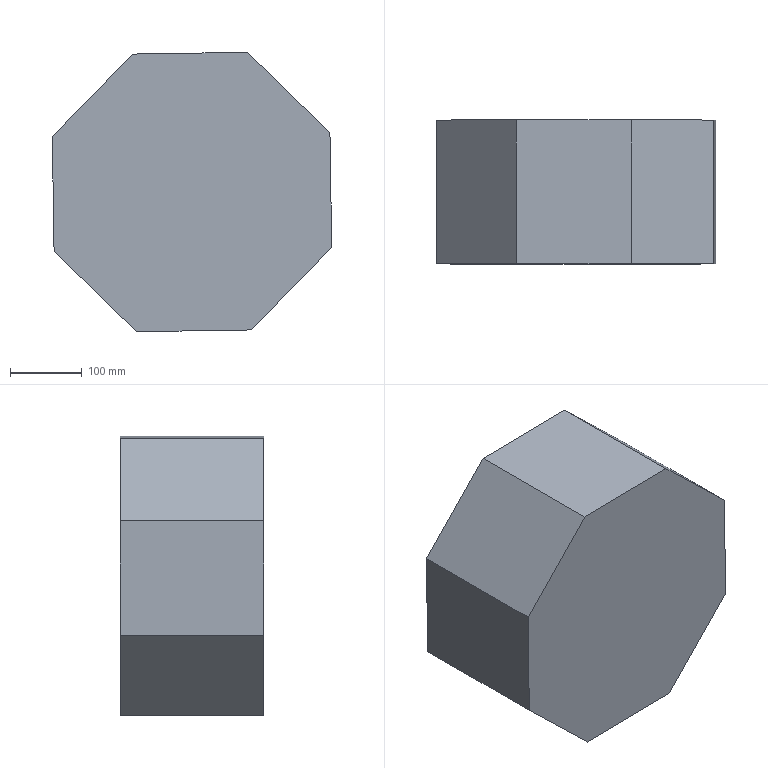Part | STEP file | octahedron 160 193.step.STEP | 1 solid | 10 faces | box 388.677 x 200 x 388.677 mm | volume 24721547 mm3 | plane 10
STEP:
#1=CARTESIAN_POINT('',(77.035,0.,194.339));
#2=VERTEX_POINT('',#1);
#3=CARTESIAN_POINT('',(191.89,0.,82.946));
#4=VERTEX_POINT('',#3);
#5=CARTESIAN_POINT('',(77.035,0.,194.339));
#6=DIRECTION('',(0.7178,0.,-0.6962));
#7=VECTOR('',#6,1000.);
#8=LINE('',#5,#7);
#9=EDGE_CURVE('',#2,#4,#8,.T.);
#10=ORIENTED_EDGE('',*,*,#9,.T.);
#11=CARTESIAN_POINT('',(191.89,200.,82.946));
#12=VERTEX_POINT('',#11);
#13=CARTESIAN_POINT('',(191.89,200.,82.946));
#14=DIRECTION('',(0.,-1.,0.));
#15=VECTOR('',#14,1000.);
#16=LINE('',#13,#15);
#17=EDGE_CURVE('',#12,#4,#16,.T.);
#18=ORIENTED_EDGE('',*,*,#17,.F.);
#19=CARTESIAN_POINT('',(77.035,200.,194.339));
#20=VERTEX_POINT('',#19);
#21=CARTESIAN_POINT('',(77.035,200.,194.339));
#22=DIRECTION('',(0.7178,0.,-0.6962));
#23=VECTOR('',#22,1000.);
#24=LINE('',#21,#23);
#25=EDGE_CURVE('',#20,#12,#24,.T.);
#26=ORIENTED_EDGE('',*,*,#25,.F.);
#27=CARTESIAN_POINT('',(77.035,200.,194.339));
#28=DIRECTION('',(0.,-1.,0.));
#29=VECTOR('',#28,1000.);
#30=LINE('',#27,#29);
#31=EDGE_CURVE('',#20,#2,#30,.T.);
#32=ORIENTED_EDGE('',*,*,#31,.T.);
#33=EDGE_LOOP('',(#10,#18,#26,#32));
#34=FACE_OUTER_BOUND('',#33,.T.);
#35=CARTESIAN_POINT('',(77.035,200.,194.339));
#36=DIRECTION('',(-0.6962,0.,-0.7178));
#37=DIRECTION('',(-0.7178,0.,0.6962));
#38=AXIS2_PLACEMENT_3D('',#35,#36,#37);
#39=PLANE('',#38);
#40=ADVANCED_FACE('',(#34),#39,.F.);
#41=CARTESIAN_POINT('',(194.339,0.,-77.035));
#42=VERTEX_POINT('',#41);
#43=CARTESIAN_POINT('',(191.89,0.,82.946));
#44=DIRECTION('',(0.0153,0.,-0.9999));
#45=VECTOR('',#44,1000.);
#46=LINE('',#43,#45);
#47=EDGE_CURVE('',#4,#42,#46,.T.);
#48=ORIENTED_EDGE('',*,*,#47,.T.);
#49=CARTESIAN_POINT('',(194.339,200.,-77.035));
#50=VERTEX_POINT('',#49);
#51=CARTESIAN_POINT('',(194.339,200.,-77.035));
#52=DIRECTION('',(0.,-1.,0.));
#53=VECTOR('',#52,1000.);
#54=LINE('',#51,#53);
#55=EDGE_CURVE('',#50,#42,#54,.T.);
#56=ORIENTED_EDGE('',*,*,#55,.F.);
#57=CARTESIAN_POINT('',(191.89,200.,82.946));
#58=DIRECTION('',(0.0153,0.,-0.9999));
#59=VECTOR('',#58,1000.);
#60=LINE('',#57,#59);
#61=EDGE_CURVE('',#12,#50,#60,.T.);
#62=ORIENTED_EDGE('',*,*,#61,.F.);
#63=ORIENTED_EDGE('',*,*,#17,.T.);
#64=EDGE_LOOP('',(#48,#56,#62,#63));
#65=FACE_OUTER_BOUND('',#64,.T.);
#66=CARTESIAN_POINT('',(191.89,200.,82.946));
#67=DIRECTION('',(-0.9999,0.,-0.0153));
#68=DIRECTION('',(-0.0153,0.,0.9999));
#69=AXIS2_PLACEMENT_3D('',#66,#67,#68);
#70=PLANE('',#69);
#71=ADVANCED_FACE('',(#65),#70,.F.);
#72=CARTESIAN_POINT('',(82.946,0.,-191.89));
#73=VERTEX_POINT('',#72);
#74=CARTESIAN_POINT('',(194.339,0.,-77.035));
#75=DIRECTION('',(-0.6962,0.,-0.7178));
#76=VECTOR('',#75,1000.);
#77=LINE('',#74,#76);
#78=EDGE_CURVE('',#42,#73,#77,.T.);
#79=ORIENTED_EDGE('',*,*,#78,.T.);
#80=CARTESIAN_POINT('',(82.946,200.,-191.89));
#81=VERTEX_POINT('',#80);
#82=CARTESIAN_POINT('',(82.946,200.,-191.89));
#83=DIRECTION('',(0.,-1.,0.));
#84=VECTOR('',#83,1000.);
#85=LINE('',#82,#84);
#86=EDGE_CURVE('',#81,#73,#85,.T.);
#87=ORIENTED_EDGE('',*,*,#86,.F.);
#88=CARTESIAN_POINT('',(194.339,200.,-77.035));
#89=DIRECTION('',(-0.6962,0.,-0.7178));
#90=VECTOR('',#89,1000.);
#91=LINE('',#88,#90);
#92=EDGE_CURVE('',#50,#81,#91,.T.);
#93=ORIENTED_EDGE('',*,*,#92,.F.);
#94=ORIENTED_EDGE('',*,*,#55,.T.);
#95=EDGE_LOOP('',(#79,#87,#93,#94));
#96=FACE_OUTER_BOUND('',#95,.T.);
#97=CARTESIAN_POINT('',(194.339,200.,-77.035));
#98=DIRECTION('',(-0.7178,0.,0.6962));
#99=DIRECTION('',(0.,1.,0.));
#100=AXIS2_PLACEMENT_3D('',#97,#98,#99);
#101=PLANE('',#100);
#102=ADVANCED_FACE('',(#96),#101,.F.);
#103=CARTESIAN_POINT('',(-77.035,0.,-194.339));
#104=VERTEX_POINT('',#103);
#105=CARTESIAN_POINT('',(82.946,0.,-191.89));
#106=DIRECTION('',(-0.9999,0.,-0.0153));
#107=VECTOR('',#106,1000.);
#108=LINE('',#105,#107);
#109=EDGE_CURVE('',#73,#104,#108,.T.);
#110=ORIENTED_EDGE('',*,*,#109,.T.);
#111=CARTESIAN_POINT('',(-77.035,200.,-194.339));
#112=VERTEX_POINT('',#111);
#113=CARTESIAN_POINT('',(-77.035,200.,-194.339));
#114=DIRECTION('',(0.,-1.,0.));
#115=VECTOR('',#114,1000.);
#116=LINE('',#113,#115);
#117=EDGE_CURVE('',#112,#104,#116,.T.);
#118=ORIENTED_EDGE('',*,*,#117,.F.);
#119=CARTESIAN_POINT('',(82.946,200.,-191.89));
#120=DIRECTION('',(-0.9999,0.,-0.0153));
#121=VECTOR('',#120,1000.);
#122=LINE('',#119,#121);
#123=EDGE_CURVE('',#81,#112,#122,.T.);
#124=ORIENTED_EDGE('',*,*,#123,.F.);
#125=ORIENTED_EDGE('',*,*,#86,.T.);
#126=EDGE_LOOP('',(#110,#118,#124,#125));
#127=FACE_OUTER_BOUND('',#126,.T.);
#128=CARTESIAN_POINT('',(82.946,200.,-191.89));
#129=DIRECTION('',(-0.0153,0.,0.9999));
#130=DIRECTION('',(0.,1.,0.));
#131=AXIS2_PLACEMENT_3D('',#128,#129,#130);
#132=PLANE('',#131);
#133=ADVANCED_FACE('',(#127),#132,.F.);
#134=CARTESIAN_POINT('',(-191.89,0.,-82.946));
#135=VERTEX_POINT('',#134);
#136=CARTESIAN_POINT('',(-77.035,0.,-194.339));
#137=DIRECTION('',(-0.7178,0.,0.6962));
#138=VECTOR('',#137,1000.);
#139=LINE('',#136,#138);
#140=EDGE_CURVE('',#104,#135,#139,.T.);
#141=ORIENTED_EDGE('',*,*,#140,.T.);
#142=CARTESIAN_POINT('',(-191.89,200.,-82.946));
#143=VERTEX_POINT('',#142);
#144=CARTESIAN_POINT('',(-191.89,200.,-82.946));
#145=DIRECTION('',(0.,-1.,0.));
#146=VECTOR('',#145,1000.);
#147=LINE('',#144,#146);
#148=EDGE_CURVE('',#143,#135,#147,.T.);
#149=ORIENTED_EDGE('',*,*,#148,.F.);
#150=CARTESIAN_POINT('',(-77.035,200.,-194.339));
#151=DIRECTION('',(-0.7178,0.,0.6962));
#152=VECTOR('',#151,1000.);
#153=LINE('',#150,#152);
#154=EDGE_CURVE('',#112,#143,#153,.T.);
#155=ORIENTED_EDGE('',*,*,#154,.F.);
#156=ORIENTED_EDGE('',*,*,#117,.T.);
#157=EDGE_LOOP('',(#141,#149,#155,#156));
#158=FACE_OUTER_BOUND('',#157,.T.);
#159=CARTESIAN_POINT('',(-77.035,200.,-194.339));
#160=DIRECTION('',(0.6962,0.,0.7178));
#161=DIRECTION('',(0.,-1.,0.));
#162=AXIS2_PLACEMENT_3D('',#159,#160,#161);
#163=PLANE('',#162);
#164=ADVANCED_FACE('',(#158),#163,.F.);
#165=CARTESIAN_POINT('',(-194.339,0.,77.035));
#166=VERTEX_POINT('',#165);
#167=CARTESIAN_POINT('',(-191.89,0.,-82.946));
#168=DIRECTION('',(-0.0153,0.,0.9999));
#169=VECTOR('',#168,1000.);
#170=LINE('',#167,#169);
#171=EDGE_CURVE('',#135,#166,#170,.T.);
#172=ORIENTED_EDGE('',*,*,#171,.T.);
#173=CARTESIAN_POINT('',(-194.339,200.,77.035));
#174=VERTEX_POINT('',#173);
#175=CARTESIAN_POINT('',(-194.339,200.,77.035));
#176=DIRECTION('',(0.,-1.,0.));
#177=VECTOR('',#176,1000.);
#178=LINE('',#175,#177);
#179=EDGE_CURVE('',#174,#166,#178,.T.);
#180=ORIENTED_EDGE('',*,*,#179,.F.);
#181=CARTESIAN_POINT('',(-191.89,200.,-82.946));
#182=DIRECTION('',(-0.0153,0.,0.9999));
#183=VECTOR('',#182,1000.);
#184=LINE('',#181,#183);
#185=EDGE_CURVE('',#143,#174,#184,.T.);
#186=ORIENTED_EDGE('',*,*,#185,.F.);
#187=ORIENTED_EDGE('',*,*,#148,.T.);
#188=EDGE_LOOP('',(#172,#180,#186,#187));
#189=FACE_OUTER_BOUND('',#188,.T.);
#190=CARTESIAN_POINT('',(-191.89,200.,-82.946));
#191=DIRECTION('',(0.9999,0.,0.0153));
#192=DIRECTION('',(0.,-1.,0.));
#193=AXIS2_PLACEMENT_3D('',#190,#191,#192);
#194=PLANE('',#193);
#195=ADVANCED_FACE('',(#189),#194,.F.);
#196=CARTESIAN_POINT('',(-82.946,0.,191.89));
#197=VERTEX_POINT('',#196);
#198=CARTESIAN_POINT('',(-194.339,0.,77.035));
#199=DIRECTION('',(0.6962,0.,0.7178));
#200=VECTOR('',#199,1000.);
#201=LINE('',#198,#200);
#202=EDGE_CURVE('',#166,#197,#201,.T.);
#203=ORIENTED_EDGE('',*,*,#202,.T.);
#204=CARTESIAN_POINT('',(-82.946,200.,191.89));
#205=VERTEX_POINT('',#204);
#206=CARTESIAN_POINT('',(-82.946,200.,191.89));
#207=DIRECTION('',(0.,-1.,0.));
#208=VECTOR('',#207,1000.);
#209=LINE('',#206,#208);
#210=EDGE_CURVE('',#205,#197,#209,.T.);
#211=ORIENTED_EDGE('',*,*,#210,.F.);
#212=CARTESIAN_POINT('',(-194.339,200.,77.035));
#213=DIRECTION('',(0.6962,0.,0.7178));
#214=VECTOR('',#213,1000.);
#215=LINE('',#212,#214);
#216=EDGE_CURVE('',#174,#205,#215,.T.);
#217=ORIENTED_EDGE('',*,*,#216,.F.);
#218=ORIENTED_EDGE('',*,*,#179,.T.);
#219=EDGE_LOOP('',(#203,#211,#217,#218));
#220=FACE_OUTER_BOUND('',#219,.T.);
#221=CARTESIAN_POINT('',(-194.339,200.,77.035));
#222=DIRECTION('',(0.7178,0.,-0.6962));
#223=DIRECTION('',(0.,-1.,0.));
#224=AXIS2_PLACEMENT_3D('',#221,#222,#223);
#225=PLANE('',#224);
#226=ADVANCED_FACE('',(#220),#225,.F.);
#227=CARTESIAN_POINT('',(-82.946,0.,191.89));
#228=DIRECTION('',(0.9999,0.,0.0153));
#229=VECTOR('',#228,1000.);
#230=LINE('',#227,#229);
#231=EDGE_CURVE('',#197,#2,#230,.T.);
#232=ORIENTED_EDGE('',*,*,#231,.T.);
#233=ORIENTED_EDGE('',*,*,#31,.F.);
#234=CARTESIAN_POINT('',(-82.946,200.,191.89));
#235=DIRECTION('',(0.9999,0.,0.0153));
#236=VECTOR('',#235,1000.);
#237=LINE('',#234,#236);
#238=EDGE_CURVE('',#205,#20,#237,.T.);
#239=ORIENTED_EDGE('',*,*,#238,.F.);
#240=ORIENTED_EDGE('',*,*,#210,.T.);
#241=EDGE_LOOP('',(#232,#233,#239,#240));
#242=FACE_OUTER_BOUND('',#241,.T.);
#243=CARTESIAN_POINT('',(-82.946,200.,191.89));
#244=DIRECTION('',(0.0153,0.,-0.9999));
#245=DIRECTION('',(0.,-1.,0.));
#246=AXIS2_PLACEMENT_3D('',#243,#244,#245);
#247=PLANE('',#246);
#248=ADVANCED_FACE('',(#242),#247,.F.);
#249=ORIENTED_EDGE('',*,*,#25,.T.);
#250=ORIENTED_EDGE('',*,*,#61,.T.);
#251=ORIENTED_EDGE('',*,*,#92,.T.);
#252=ORIENTED_EDGE('',*,*,#123,.T.);
#253=ORIENTED_EDGE('',*,*,#154,.T.);
#254=ORIENTED_EDGE('',*,*,#185,.T.);
#255=ORIENTED_EDGE('',*,*,#216,.T.);
#256=ORIENTED_EDGE('',*,*,#238,.T.);
#257=EDGE_LOOP('',(#249,#250,#251,#252,#253,#254,#255,#256));
#258=FACE_OUTER_BOUND('',#257,.T.);
#259=CARTESIAN_POINT('',(0.,200.,0.));
#260=DIRECTION('',(0.,1.,0.));
#261=DIRECTION('',(1.,0.,0.));
#262=AXIS2_PLACEMENT_3D('',#259,#260,#261);
#263=PLANE('',#262);
#264=ADVANCED_FACE('',(#258),#263,.T.);
#265=ORIENTED_EDGE('',*,*,#9,.F.);
#266=ORIENTED_EDGE('',*,*,#231,.F.);
#267=ORIENTED_EDGE('',*,*,#202,.F.);
#268=ORIENTED_EDGE('',*,*,#171,.F.);
#269=ORIENTED_EDGE('',*,*,#140,.F.);
#270=ORIENTED_EDGE('',*,*,#109,.F.);
#271=ORIENTED_EDGE('',*,*,#78,.F.);
#272=ORIENTED_EDGE('',*,*,#47,.F.);
#273=EDGE_LOOP('',(#265,#266,#267,#268,#269,#270,#271,#272));
#274=FACE_OUTER_BOUND('',#273,.T.);
#275=CARTESIAN_POINT('',(0.,0.,0.));
#276=DIRECTION('',(0.,1.,0.));
#277=DIRECTION('',(1.,0.,0.));
#278=AXIS2_PLACEMENT_3D('',#275,#276,#277);
#279=PLANE('',#278);
#280=ADVANCED_FACE('',(#274),#279,.F.);
#281=CLOSED_SHELL('',(#40,#71,#102,#133,#164,#195,#226,#248,#264,#280));
#282=MANIFOLD_SOLID_BREP('',#281);
#283=CARTESIAN_POINT('',(0.,0.,0.));
#284=DIRECTION('',(0.,0.,1.));
#285=DIRECTION('',(1.,0.,0.));
#286=AXIS2_PLACEMENT_3D('',#283,#284,#285);
#287=(LENGTH_UNIT()NAMED_UNIT(*)SI_UNIT(.MILLI.,.METRE.));
#288=UNCERTAINTY_MEASURE_WITH_UNIT(LENGTH_MEASURE(0.00001),#287,'','');
#289=(NAMED_UNIT(*)PLANE_ANGLE_UNIT()SI_UNIT($,.RADIAN.));
#290=(NAMED_UNIT(*)SI_UNIT($,.STERADIAN.)SOLID_ANGLE_UNIT());
#291=(GEOMETRIC_REPRESENTATION_CONTEXT(3)GLOBAL_UNCERTAINTY_ASSIGNED_CONTEXT((#288))GLOBAL_UNIT_ASSIGNED_CONTEXT((#287,#289,#290))REPRESENTATION_CONTEXT('',''));
#292=ADVANCED_BREP_SHAPE_REPRESENTATION('',(#282,#286),#291);